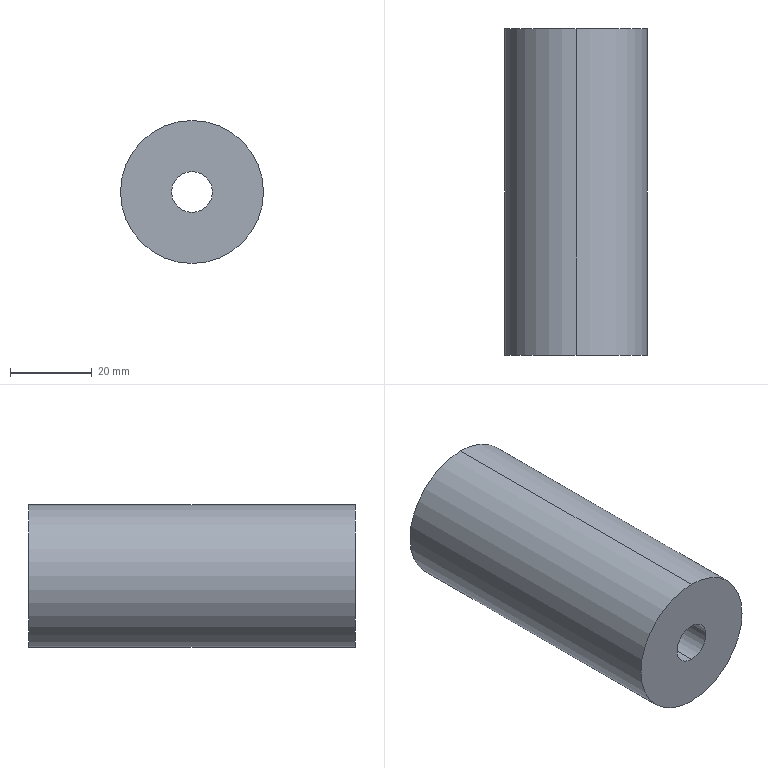Part | STEP file | 1 solid | 6 faces | box 35 x 80 x 35 mm | volume 70686 mm3 | cylinder 4 | plane 2 | commonest cylinder face diameters 10 x2 35 x2
STEP:
#1=CARTESIAN_POINT('',(0.,0.,0.));
#2=DIRECTION('',(0.,0.,1.));
#3=DIRECTION('',(1.,0.,0.));
#4=AXIS2_PLACEMENT_3D('',#1,#2,#3);
#5=CARTESIAN_POINT('',(0.,0.,17.5));
#6=VERTEX_POINT('',#5);
#7=CARTESIAN_POINT('',(0.,0.,-17.5));
#8=VERTEX_POINT('',#7);
#9=CARTESIAN_POINT('',(0.,0.,0.));
#10=DIRECTION('',(0.,1.,0.));
#11=DIRECTION('',(0.,0.,1.));
#12=AXIS2_PLACEMENT_3D('',#9,#10,#11);
#13=CIRCLE('',#12,17.5);
#14=CARTESIAN_POINT('',(0.,0.,0.));
#15=DIRECTION('',(0.,1.,0.));
#16=DIRECTION('',(0.,0.,1.));
#17=AXIS2_PLACEMENT_3D('',#14,#15,#16);
#18=CYLINDRICAL_SURFACE('',#17,17.5);
#19=CARTESIAN_POINT('',(0.,0.));
#20=DIRECTION('',(1.,0.));
#21=VECTOR('',#20,1.);
#22=LINE('',#19,#21);
#23=(GEOMETRIC_REPRESENTATION_CONTEXT(2)PARAMETRIC_REPRESENTATION_CONTEXT()REPRESENTATION_CONTEXT('',''));
#24=DEFINITIONAL_REPRESENTATION('',(#22),#23);
#25=PCURVE('',#18,#24);
#26=CARTESIAN_POINT('',(0.,0.,0.));
#27=DIRECTION('',(0.,1.,0.));
#28=DIRECTION('',(0.,0.,1.));
#29=AXIS2_PLACEMENT_3D('',#26,#27,#28);
#30=PLANE('',#29);
#31=CARTESIAN_POINT('',(0.,0.));
#32=DIRECTION('',(1.,0.));
#33=AXIS2_PLACEMENT_2D('',#31,#32);
#34=CIRCLE('',#33,17.5);
#35=(GEOMETRIC_REPRESENTATION_CONTEXT(2)PARAMETRIC_REPRESENTATION_CONTEXT()REPRESENTATION_CONTEXT('',''));
#36=DEFINITIONAL_REPRESENTATION('',(#34),#35);
#37=PCURVE('',#30,#36);
#38=SURFACE_CURVE('',#13,(#25,#37),.PCURVE_S1.);
#39=EDGE_CURVE('',#6,#8,#38,.T.);
#40=ORIENTED_EDGE('',*,*,#39,.T.);
#41=CARTESIAN_POINT('',(0.,80.,-17.5));
#42=VERTEX_POINT('',#41);
#43=CARTESIAN_POINT('',(0.,0.,-17.5));
#44=DIRECTION('',(0.,1.,0.));
#45=VECTOR('',#44,1.);
#46=LINE('',#43,#45);
#47=CARTESIAN_POINT('',(3.142,0.));
#48=DIRECTION('',(0.,1.));
#49=VECTOR('',#48,1.);
#50=LINE('',#47,#49);
#51=(GEOMETRIC_REPRESENTATION_CONTEXT(2)PARAMETRIC_REPRESENTATION_CONTEXT()REPRESENTATION_CONTEXT('',''));
#52=DEFINITIONAL_REPRESENTATION('',(#50),#51);
#53=PCURVE('',#18,#52);
#54=CARTESIAN_POINT('',(0.,0.,0.));
#55=DIRECTION('',(0.,1.,0.));
#56=DIRECTION('',(0.,0.,1.));
#57=AXIS2_PLACEMENT_3D('',#54,#55,#56);
#58=CYLINDRICAL_SURFACE('',#57,17.5);
#59=CARTESIAN_POINT('',(3.142,0.));
#60=DIRECTION('',(0.,1.));
#61=VECTOR('',#60,1.);
#62=LINE('',#59,#61);
#63=(GEOMETRIC_REPRESENTATION_CONTEXT(2)PARAMETRIC_REPRESENTATION_CONTEXT()REPRESENTATION_CONTEXT('',''));
#64=DEFINITIONAL_REPRESENTATION('',(#62),#63);
#65=PCURVE('',#58,#64);
#66=SURFACE_CURVE('',#46,(#53,#65),.PCURVE_S1.);
#67=EDGE_CURVE('',#8,#42,#66,.T.);
#68=ORIENTED_EDGE('',*,*,#67,.T.);
#69=CARTESIAN_POINT('',(0.,80.,17.5));
#70=VERTEX_POINT('',#69);
#71=CARTESIAN_POINT('',(0.,80.,0.));
#72=DIRECTION('',(0.,-1.,0.));
#73=DIRECTION('',(0.,0.,1.));
#74=AXIS2_PLACEMENT_3D('',#71,#72,#73);
#75=CIRCLE('',#74,17.5);
#76=CARTESIAN_POINT('',(6.283,80.));
#77=DIRECTION('',(-1.,0.));
#78=VECTOR('',#77,1.);
#79=LINE('',#76,#78);
#80=(GEOMETRIC_REPRESENTATION_CONTEXT(2)PARAMETRIC_REPRESENTATION_CONTEXT()REPRESENTATION_CONTEXT('',''));
#81=DEFINITIONAL_REPRESENTATION('',(#79),#80);
#82=PCURVE('',#18,#81);
#83=CARTESIAN_POINT('',(0.,80.,0.));
#84=DIRECTION('',(0.,1.,0.));
#85=DIRECTION('',(0.,0.,1.));
#86=AXIS2_PLACEMENT_3D('',#83,#84,#85);
#87=PLANE('',#86);
#88=CARTESIAN_POINT('',(17.5,0.));
#89=CARTESIAN_POINT('',(17.5,-30.311));
#90=CARTESIAN_POINT('',(-8.75,-15.155));
#91=CARTESIAN_POINT('',(-35.,0.));
#92=CARTESIAN_POINT('',(-8.75,15.155));
#93=CARTESIAN_POINT('',(17.5,30.311));
#94=CARTESIAN_POINT('',(17.5,0.));
#95=(BOUNDED_CURVE()B_SPLINE_CURVE(2,(#88,#89,#90,#91,#92,#93,#94),.UNSPECIFIED.,.T.,.F.)B_SPLINE_CURVE_WITH_KNOTS((1,2,2,2,2,1),(-2.094,0.,2.094,4.189,6.283,8.378),.UNSPECIFIED.)CURVE()GEOMETRIC_REPRESENTATION_ITEM()RATIONAL_B_SPLINE_CURVE((1.,0.5,1.,0.5,1.,0.5,1.))REPRESENTATION_ITEM(''));
#96=(GEOMETRIC_REPRESENTATION_CONTEXT(2)PARAMETRIC_REPRESENTATION_CONTEXT()REPRESENTATION_CONTEXT('',''));
#97=DEFINITIONAL_REPRESENTATION('',(#95),#96);
#98=PCURVE('',#87,#97);
#99=SURFACE_CURVE('',#75,(#82,#98),.PCURVE_S1.);
#100=EDGE_CURVE('',#42,#70,#99,.T.);
#101=ORIENTED_EDGE('',*,*,#100,.T.);
#102=CARTESIAN_POINT('',(0.,0.,17.5));
#103=DIRECTION('',(0.,1.,0.));
#104=VECTOR('',#103,1.);
#105=LINE('',#102,#104);
#106=CARTESIAN_POINT('',(0.,0.));
#107=DIRECTION('',(0.,1.));
#108=VECTOR('',#107,1.);
#109=LINE('',#106,#108);
#110=(GEOMETRIC_REPRESENTATION_CONTEXT(2)PARAMETRIC_REPRESENTATION_CONTEXT()REPRESENTATION_CONTEXT('',''));
#111=DEFINITIONAL_REPRESENTATION('',(#109),#110);
#112=PCURVE('',#18,#111);
#113=CARTESIAN_POINT('',(6.283,0.));
#114=DIRECTION('',(0.,1.));
#115=VECTOR('',#114,1.);
#116=LINE('',#113,#115);
#117=(GEOMETRIC_REPRESENTATION_CONTEXT(2)PARAMETRIC_REPRESENTATION_CONTEXT()REPRESENTATION_CONTEXT('',''));
#118=DEFINITIONAL_REPRESENTATION('',(#116),#117);
#119=PCURVE('',#58,#118);
#120=SURFACE_CURVE('',#105,(#112,#119),.PCURVE_S1.);
#121=EDGE_CURVE('',#6,#70,#120,.T.);
#122=ORIENTED_EDGE('',*,*,#121,.F.);
#123=EDGE_LOOP('',(#40,#68,#101,#122));
#124=FACE_BOUND('',#123,.T.);
#125=ADVANCED_FACE('',(#124),#18,.T.);
#126=CARTESIAN_POINT('',(0.,0.,5.));
#127=VERTEX_POINT('',#126);
#128=CARTESIAN_POINT('',(0.,80.,5.));
#129=VERTEX_POINT('',#128);
#130=CARTESIAN_POINT('',(0.,0.,5.));
#131=DIRECTION('',(0.,1.,0.));
#132=VECTOR('',#131,1.);
#133=LINE('',#130,#132);
#134=CARTESIAN_POINT('',(0.,0.,0.));
#135=DIRECTION('',(0.,1.,0.));
#136=DIRECTION('',(0.,0.,1.));
#137=AXIS2_PLACEMENT_3D('',#134,#135,#136);
#138=CYLINDRICAL_SURFACE('',#137,5.);
#139=CARTESIAN_POINT('',(6.283,0.));
#140=DIRECTION('',(0.,1.));
#141=VECTOR('',#140,1.);
#142=LINE('',#139,#141);
#143=(GEOMETRIC_REPRESENTATION_CONTEXT(2)PARAMETRIC_REPRESENTATION_CONTEXT()REPRESENTATION_CONTEXT('',''));
#144=DEFINITIONAL_REPRESENTATION('',(#142),#143);
#145=PCURVE('',#138,#144);
#146=CARTESIAN_POINT('',(0.,0.,0.));
#147=DIRECTION('',(0.,1.,0.));
#148=DIRECTION('',(0.,0.,1.));
#149=AXIS2_PLACEMENT_3D('',#146,#147,#148);
#150=CYLINDRICAL_SURFACE('',#149,5.);
#151=CARTESIAN_POINT('',(0.,0.));
#152=DIRECTION('',(0.,1.));
#153=VECTOR('',#152,1.);
#154=LINE('',#151,#153);
#155=(GEOMETRIC_REPRESENTATION_CONTEXT(2)PARAMETRIC_REPRESENTATION_CONTEXT()REPRESENTATION_CONTEXT('',''));
#156=DEFINITIONAL_REPRESENTATION('',(#154),#155);
#157=PCURVE('',#150,#156);
#158=SURFACE_CURVE('',#133,(#145,#157),.PCURVE_S1.);
#159=EDGE_CURVE('',#127,#129,#158,.T.);
#160=ORIENTED_EDGE('',*,*,#159,.T.);
#161=CARTESIAN_POINT('',(0.,80.,-5.));
#162=VERTEX_POINT('',#161);
#163=CARTESIAN_POINT('',(0.,80.,0.));
#164=DIRECTION('',(0.,-1.,0.));
#165=DIRECTION('',(0.,0.,1.));
#166=AXIS2_PLACEMENT_3D('',#163,#164,#165);
#167=CIRCLE('',#166,5.);
#168=CARTESIAN_POINT('',(6.283,80.));
#169=DIRECTION('',(-1.,0.));
#170=VECTOR('',#169,1.);
#171=LINE('',#168,#170);
#172=(GEOMETRIC_REPRESENTATION_CONTEXT(2)PARAMETRIC_REPRESENTATION_CONTEXT()REPRESENTATION_CONTEXT('',''));
#173=DEFINITIONAL_REPRESENTATION('',(#171),#172);
#174=PCURVE('',#138,#173);
#175=CARTESIAN_POINT('',(5.,0.));
#176=CARTESIAN_POINT('',(5.,-8.66));
#177=CARTESIAN_POINT('',(-2.5,-4.33));
#178=CARTESIAN_POINT('',(-10.,0.));
#179=CARTESIAN_POINT('',(-2.5,4.33));
#180=CARTESIAN_POINT('',(5.,8.66));
#181=CARTESIAN_POINT('',(5.,0.));
#182=(BOUNDED_CURVE()B_SPLINE_CURVE(2,(#175,#176,#177,#178,#179,#180,#181),.UNSPECIFIED.,.T.,.F.)B_SPLINE_CURVE_WITH_KNOTS((1,2,2,2,2,1),(-2.094,0.,2.094,4.189,6.283,8.378),.UNSPECIFIED.)CURVE()GEOMETRIC_REPRESENTATION_ITEM()RATIONAL_B_SPLINE_CURVE((1.,0.5,1.,0.5,1.,0.5,1.))REPRESENTATION_ITEM(''));
#183=(GEOMETRIC_REPRESENTATION_CONTEXT(2)PARAMETRIC_REPRESENTATION_CONTEXT()REPRESENTATION_CONTEXT('',''));
#184=DEFINITIONAL_REPRESENTATION('',(#182),#183);
#185=PCURVE('',#87,#184);
#186=SURFACE_CURVE('',#167,(#174,#185),.PCURVE_S1.);
#187=EDGE_CURVE('',#129,#162,#186,.T.);
#188=ORIENTED_EDGE('',*,*,#187,.T.);
#189=CARTESIAN_POINT('',(0.,0.,-5.));
#190=VERTEX_POINT('',#189);
#191=CARTESIAN_POINT('',(0.,0.,-5.));
#192=DIRECTION('',(0.,1.,0.));
#193=VECTOR('',#192,1.);
#194=LINE('',#191,#193);
#195=CARTESIAN_POINT('',(3.142,0.));
#196=DIRECTION('',(0.,1.));
#197=VECTOR('',#196,1.);
#198=LINE('',#195,#197);
#199=(GEOMETRIC_REPRESENTATION_CONTEXT(2)PARAMETRIC_REPRESENTATION_CONTEXT()REPRESENTATION_CONTEXT('',''));
#200=DEFINITIONAL_REPRESENTATION('',(#198),#199);
#201=PCURVE('',#138,#200);
#202=CARTESIAN_POINT('',(3.142,0.));
#203=DIRECTION('',(0.,1.));
#204=VECTOR('',#203,1.);
#205=LINE('',#202,#204);
#206=(GEOMETRIC_REPRESENTATION_CONTEXT(2)PARAMETRIC_REPRESENTATION_CONTEXT()REPRESENTATION_CONTEXT('',''));
#207=DEFINITIONAL_REPRESENTATION('',(#205),#206);
#208=PCURVE('',#150,#207);
#209=SURFACE_CURVE('',#194,(#201,#208),.PCURVE_S1.);
#210=EDGE_CURVE('',#190,#162,#209,.T.);
#211=ORIENTED_EDGE('',*,*,#210,.F.);
#212=CARTESIAN_POINT('',(0.,0.,0.));
#213=DIRECTION('',(0.,-1.,0.));
#214=DIRECTION('',(0.,0.,1.));
#215=AXIS2_PLACEMENT_3D('',#212,#213,#214);
#216=CIRCLE('',#215,5.);
#217=CARTESIAN_POINT('',(6.283,0.));
#218=DIRECTION('',(-1.,0.));
#219=VECTOR('',#218,1.);
#220=LINE('',#217,#219);
#221=(GEOMETRIC_REPRESENTATION_CONTEXT(2)PARAMETRIC_REPRESENTATION_CONTEXT()REPRESENTATION_CONTEXT('',''));
#222=DEFINITIONAL_REPRESENTATION('',(#220),#221);
#223=PCURVE('',#138,#222);
#224=CARTESIAN_POINT('',(5.,0.));
#225=CARTESIAN_POINT('',(5.,-8.66));
#226=CARTESIAN_POINT('',(-2.5,-4.33));
#227=CARTESIAN_POINT('',(-10.,0.));
#228=CARTESIAN_POINT('',(-2.5,4.33));
#229=CARTESIAN_POINT('',(5.,8.66));
#230=CARTESIAN_POINT('',(5.,0.));
#231=(BOUNDED_CURVE()B_SPLINE_CURVE(2,(#224,#225,#226,#227,#228,#229,#230),.UNSPECIFIED.,.T.,.F.)B_SPLINE_CURVE_WITH_KNOTS((1,2,2,2,2,1),(-2.094,0.,2.094,4.189,6.283,8.378),.UNSPECIFIED.)CURVE()GEOMETRIC_REPRESENTATION_ITEM()RATIONAL_B_SPLINE_CURVE((1.,0.5,1.,0.5,1.,0.5,1.))REPRESENTATION_ITEM(''));
#232=(GEOMETRIC_REPRESENTATION_CONTEXT(2)PARAMETRIC_REPRESENTATION_CONTEXT()REPRESENTATION_CONTEXT('',''));
#233=DEFINITIONAL_REPRESENTATION('',(#231),#232);
#234=PCURVE('',#30,#233);
#235=SURFACE_CURVE('',#216,(#223,#234),.PCURVE_S1.);
#236=EDGE_CURVE('',#127,#190,#235,.T.);
#237=ORIENTED_EDGE('',*,*,#236,.F.);
#238=EDGE_LOOP('',(#160,#188,#211,#237));
#239=FACE_BOUND('',#238,.F.);
#240=ADVANCED_FACE('',(#239),#138,.F.);
#241=ORIENTED_EDGE('',*,*,#67,.F.);
#242=CARTESIAN_POINT('',(0.,0.,0.));
#243=DIRECTION('',(0.,1.,0.));
#244=DIRECTION('',(0.,0.,1.));
#245=AXIS2_PLACEMENT_3D('',#242,#243,#244);
#246=CIRCLE('',#245,17.5);
#247=CARTESIAN_POINT('',(0.,0.));
#248=DIRECTION('',(1.,0.));
#249=VECTOR('',#248,1.);
#250=LINE('',#247,#249);
#251=(GEOMETRIC_REPRESENTATION_CONTEXT(2)PARAMETRIC_REPRESENTATION_CONTEXT()REPRESENTATION_CONTEXT('',''));
#252=DEFINITIONAL_REPRESENTATION('',(#250),#251);
#253=PCURVE('',#58,#252);
#254=CARTESIAN_POINT('',(0.,0.));
#255=DIRECTION('',(1.,0.));
#256=AXIS2_PLACEMENT_2D('',#254,#255);
#257=CIRCLE('',#256,17.5);
#258=(GEOMETRIC_REPRESENTATION_CONTEXT(2)PARAMETRIC_REPRESENTATION_CONTEXT()REPRESENTATION_CONTEXT('',''));
#259=DEFINITIONAL_REPRESENTATION('',(#257),#258);
#260=PCURVE('',#30,#259);
#261=SURFACE_CURVE('',#246,(#253,#260),.PCURVE_S1.);
#262=EDGE_CURVE('',#8,#6,#261,.T.);
#263=ORIENTED_EDGE('',*,*,#262,.T.);
#264=ORIENTED_EDGE('',*,*,#121,.T.);
#265=CARTESIAN_POINT('',(0.,80.,0.));
#266=DIRECTION('',(0.,-1.,0.));
#267=DIRECTION('',(0.,0.,1.));
#268=AXIS2_PLACEMENT_3D('',#265,#266,#267);
#269=CIRCLE('',#268,17.5);
#270=CARTESIAN_POINT('',(6.283,80.));
#271=DIRECTION('',(-1.,0.));
#272=VECTOR('',#271,1.);
#273=LINE('',#270,#272);
#274=(GEOMETRIC_REPRESENTATION_CONTEXT(2)PARAMETRIC_REPRESENTATION_CONTEXT()REPRESENTATION_CONTEXT('',''));
#275=DEFINITIONAL_REPRESENTATION('',(#273),#274);
#276=PCURVE('',#58,#275);
#277=CARTESIAN_POINT('',(17.5,0.));
#278=CARTESIAN_POINT('',(17.5,-30.311));
#279=CARTESIAN_POINT('',(-8.75,-15.155));
#280=CARTESIAN_POINT('',(-35.,0.));
#281=CARTESIAN_POINT('',(-8.75,15.155));
#282=CARTESIAN_POINT('',(17.5,30.311));
#283=CARTESIAN_POINT('',(17.5,0.));
#284=(BOUNDED_CURVE()B_SPLINE_CURVE(2,(#277,#278,#279,#280,#281,#282,#283),.UNSPECIFIED.,.T.,.F.)B_SPLINE_CURVE_WITH_KNOTS((1,2,2,2,2,1),(-2.094,0.,2.094,4.189,6.283,8.378),.UNSPECIFIED.)CURVE()GEOMETRIC_REPRESENTATION_ITEM()RATIONAL_B_SPLINE_CURVE((1.,0.5,1.,0.5,1.,0.5,1.))REPRESENTATION_ITEM(''));
#285=(GEOMETRIC_REPRESENTATION_CONTEXT(2)PARAMETRIC_REPRESENTATION_CONTEXT()REPRESENTATION_CONTEXT('',''));
#286=DEFINITIONAL_REPRESENTATION('',(#284),#285);
#287=PCURVE('',#87,#286);
#288=SURFACE_CURVE('',#269,(#276,#287),.PCURVE_S1.);
#289=EDGE_CURVE('',#70,#42,#288,.T.);
#290=ORIENTED_EDGE('',*,*,#289,.T.);
#291=EDGE_LOOP('',(#241,#263,#264,#290));
#292=FACE_BOUND('',#291,.T.);
#293=ADVANCED_FACE('',(#292),#58,.T.);
#294=ORIENTED_EDGE('',*,*,#39,.F.);
#295=ORIENTED_EDGE('',*,*,#262,.F.);
#296=EDGE_LOOP('',(#294,#295));
#297=FACE_BOUND('',#296,.T.);
#298=ORIENTED_EDGE('',*,*,#236,.F.);
#299=CARTESIAN_POINT('',(0.,0.,0.));
#300=DIRECTION('',(0.,-1.,0.));
#301=DIRECTION('',(0.,0.,1.));
#302=AXIS2_PLACEMENT_3D('',#299,#300,#301);
#303=CIRCLE('',#302,5.);
#304=CARTESIAN_POINT('',(5.,0.));
#305=CARTESIAN_POINT('',(5.,-8.66));
#306=CARTESIAN_POINT('',(-2.5,-4.33));
#307=CARTESIAN_POINT('',(-10.,0.));
#308=CARTESIAN_POINT('',(-2.5,4.33));
#309=CARTESIAN_POINT('',(5.,8.66));
#310=CARTESIAN_POINT('',(5.,0.));
#311=(BOUNDED_CURVE()B_SPLINE_CURVE(2,(#304,#305,#306,#307,#308,#309,#310),.UNSPECIFIED.,.T.,.F.)B_SPLINE_CURVE_WITH_KNOTS((1,2,2,2,2,1),(-2.094,0.,2.094,4.189,6.283,8.378),.UNSPECIFIED.)CURVE()GEOMETRIC_REPRESENTATION_ITEM()RATIONAL_B_SPLINE_CURVE((1.,0.5,1.,0.5,1.,0.5,1.))REPRESENTATION_ITEM(''));
#312=(GEOMETRIC_REPRESENTATION_CONTEXT(2)PARAMETRIC_REPRESENTATION_CONTEXT()REPRESENTATION_CONTEXT('',''));
#313=DEFINITIONAL_REPRESENTATION('',(#311),#312);
#314=PCURVE('',#30,#313);
#315=CARTESIAN_POINT('',(6.283,0.));
#316=DIRECTION('',(-1.,0.));
#317=VECTOR('',#316,1.);
#318=LINE('',#315,#317);
#319=(GEOMETRIC_REPRESENTATION_CONTEXT(2)PARAMETRIC_REPRESENTATION_CONTEXT()REPRESENTATION_CONTEXT('',''));
#320=DEFINITIONAL_REPRESENTATION('',(#318),#319);
#321=PCURVE('',#150,#320);
#322=SURFACE_CURVE('',#303,(#314,#321),.PCURVE_S1.);
#323=EDGE_CURVE('',#190,#127,#322,.T.);
#324=ORIENTED_EDGE('',*,*,#323,.F.);
#325=EDGE_LOOP('',(#298,#324));
#326=FACE_BOUND('',#325,.T.);
#327=ADVANCED_FACE('',(#297,#326),#30,.F.);
#328=ORIENTED_EDGE('',*,*,#289,.F.);
#329=ORIENTED_EDGE('',*,*,#100,.F.);
#330=EDGE_LOOP('',(#328,#329));
#331=FACE_BOUND('',#330,.T.);
#332=ORIENTED_EDGE('',*,*,#187,.T.);
#333=CARTESIAN_POINT('',(0.,80.,0.));
#334=DIRECTION('',(0.,-1.,0.));
#335=DIRECTION('',(0.,0.,1.));
#336=AXIS2_PLACEMENT_3D('',#333,#334,#335);
#337=CIRCLE('',#336,5.);
#338=CARTESIAN_POINT('',(5.,0.));
#339=CARTESIAN_POINT('',(5.,-8.66));
#340=CARTESIAN_POINT('',(-2.5,-4.33));
#341=CARTESIAN_POINT('',(-10.,0.));
#342=CARTESIAN_POINT('',(-2.5,4.33));
#343=CARTESIAN_POINT('',(5.,8.66));
#344=CARTESIAN_POINT('',(5.,0.));
#345=(BOUNDED_CURVE()B_SPLINE_CURVE(2,(#338,#339,#340,#341,#342,#343,#344),.UNSPECIFIED.,.T.,.F.)B_SPLINE_CURVE_WITH_KNOTS((1,2,2,2,2,1),(-2.094,0.,2.094,4.189,6.283,8.378),.UNSPECIFIED.)CURVE()GEOMETRIC_REPRESENTATION_ITEM()RATIONAL_B_SPLINE_CURVE((1.,0.5,1.,0.5,1.,0.5,1.))REPRESENTATION_ITEM(''));
#346=(GEOMETRIC_REPRESENTATION_CONTEXT(2)PARAMETRIC_REPRESENTATION_CONTEXT()REPRESENTATION_CONTEXT('',''));
#347=DEFINITIONAL_REPRESENTATION('',(#345),#346);
#348=PCURVE('',#87,#347);
#349=CARTESIAN_POINT('',(6.283,80.));
#350=DIRECTION('',(-1.,0.));
#351=VECTOR('',#350,1.);
#352=LINE('',#349,#351);
#353=(GEOMETRIC_REPRESENTATION_CONTEXT(2)PARAMETRIC_REPRESENTATION_CONTEXT()REPRESENTATION_CONTEXT('',''));
#354=DEFINITIONAL_REPRESENTATION('',(#352),#353);
#355=PCURVE('',#150,#354);
#356=SURFACE_CURVE('',#337,(#348,#355),.PCURVE_S1.);
#357=EDGE_CURVE('',#162,#129,#356,.T.);
#358=ORIENTED_EDGE('',*,*,#357,.T.);
#359=EDGE_LOOP('',(#332,#358));
#360=FACE_BOUND('',#359,.T.);
#361=ADVANCED_FACE('',(#331,#360),#87,.T.);
#362=ORIENTED_EDGE('',*,*,#357,.T.);
#363=ORIENTED_EDGE('',*,*,#159,.F.);
#364=ORIENTED_EDGE('',*,*,#323,.F.);
#365=ORIENTED_EDGE('',*,*,#210,.T.);
#366=EDGE_LOOP('',(#362,#363,#364,#365));
#367=FACE_BOUND('',#366,.F.);
#368=ADVANCED_FACE('',(#367),#150,.F.);
#369=CLOSED_SHELL('',(#125,#240,#293,#327,#361,#368));
#370=MANIFOLD_SOLID_BREP('',#369);
#371=(LENGTH_UNIT()NAMED_UNIT(*)SI_UNIT(.MILLI.,.METRE.));
#372=UNCERTAINTY_MEASURE_WITH_UNIT(LENGTH_MEASURE(0.0000001),#371,'','');
#373=(NAMED_UNIT(*)PLANE_ANGLE_UNIT()SI_UNIT($,.RADIAN.));
#374=(NAMED_UNIT(*)SI_UNIT($,.STERADIAN.)SOLID_ANGLE_UNIT());
#375=(GEOMETRIC_REPRESENTATION_CONTEXT(3)GLOBAL_UNCERTAINTY_ASSIGNED_CONTEXT((#372))GLOBAL_UNIT_ASSIGNED_CONTEXT((#371,#373,#374))REPRESENTATION_CONTEXT('',''));
#376=ADVANCED_BREP_SHAPE_REPRESENTATION('',(#4,#370),#375);